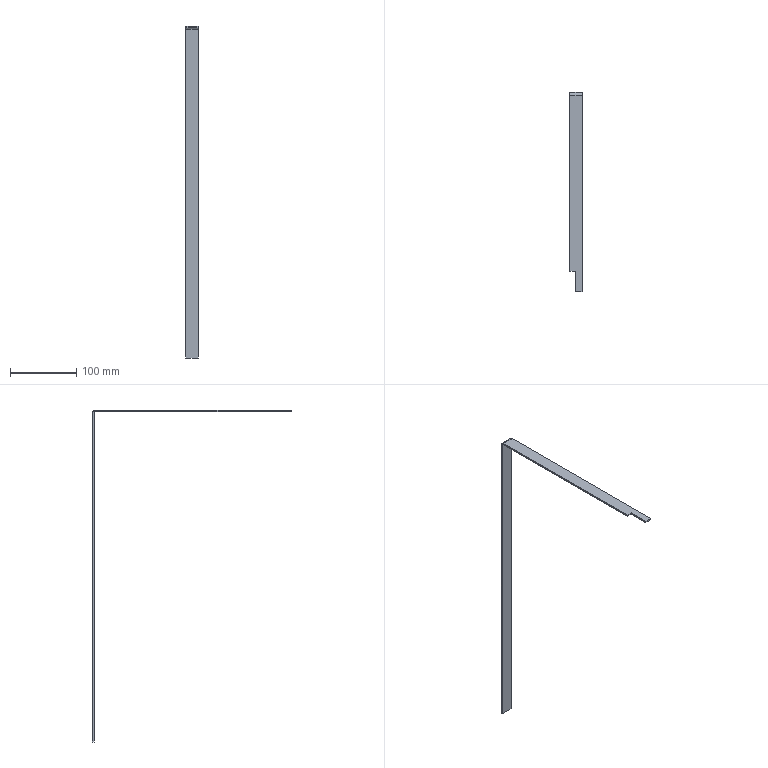Part | NX | features solid 2 | 1 solid | 12 faces | box 18.5 x 301.6 x 502.6 mm | volume 36384 mm3 | plane 10 | cylinder 2 | commonest cylinder face diameters 5 x1 10 x1
STEP:
#1=CARTESIAN_POINT('',(1098.,87.,522.6));
#2=VERTEX_POINT('',#1);
#3=CARTESIAN_POINT('',(1098.,87.,520.1));
#4=VERTEX_POINT('',#3);
#5=CARTESIAN_POINT('',(1098.,87.,520.1));
#6=DIRECTION('',(0.,0.,-1.));
#7=VECTOR('',#6,1000.);
#8=LINE('',#5,#7);
#9=EDGE_CURVE('',#2,#4,#8,.T.);
#10=ORIENTED_EDGE('',*,*,#9,.T.);
#11=CARTESIAN_POINT('',(1098.,56.,520.1));
#12=VERTEX_POINT('',#11);
#13=CARTESIAN_POINT('',(1098.,72.,520.1));
#14=DIRECTION('',(0.,1.,0.));
#15=VECTOR('',#14,1000.);
#16=LINE('',#13,#15);
#17=EDGE_CURVE('',#12,#4,#16,.T.);
#18=ORIENTED_EDGE('',*,*,#17,.F.);
#19=CARTESIAN_POINT('',(1098.,56.,522.6));
#20=VERTEX_POINT('',#19);
#21=CARTESIAN_POINT('',(1098.,56.,520.1));
#22=DIRECTION('',(0.,0.,-1.));
#23=VECTOR('',#22,1000.);
#24=LINE('',#21,#23);
#25=EDGE_CURVE('',#20,#12,#24,.T.);
#26=ORIENTED_EDGE('',*,*,#25,.F.);
#27=CARTESIAN_POINT('',(1098.,72.,522.6));
#28=DIRECTION('',(0.,1.,0.));
#29=VECTOR('',#28,1000.);
#30=LINE('',#27,#29);
#31=EDGE_CURVE('',#20,#2,#30,.T.);
#32=ORIENTED_EDGE('',*,*,#31,.T.);
#33=EDGE_LOOP('',(#10,#18,#26,#32));
#34=FACE_BOUND('',#33,.T.);
#35=CARTESIAN_POINT('',(1098.,72.,520.1));
#36=DIRECTION('',(-1.,0.,0.));
#37=DIRECTION('',(0.,0.,1.));
#38=AXIS2_PLACEMENT_3D('',#35,#36,#37);
#39=PLANE('',#38);
#40=ADVANCED_FACE('',(#34),#39,.T.);
#41=CARTESIAN_POINT('',(1090.,87.,522.6));
#42=VERTEX_POINT('',#41);
#43=CARTESIAN_POINT('',(1090.,87.,520.1));
#44=VERTEX_POINT('',#43);
#45=CARTESIAN_POINT('',(1090.,87.,520.1));
#46=DIRECTION('',(0.,0.,-1.));
#47=VECTOR('',#46,1000.);
#48=LINE('',#45,#47);
#49=EDGE_CURVE('',#42,#44,#48,.T.);
#50=ORIENTED_EDGE('',*,*,#49,.T.);
#51=CARTESIAN_POINT('',(1090.,87.,520.1));
#52=DIRECTION('',(-1.,0.,0.));
#53=VECTOR('',#52,1000.);
#54=LINE('',#51,#53);
#55=EDGE_CURVE('',#4,#44,#54,.T.);
#56=ORIENTED_EDGE('',*,*,#55,.F.);
#57=ORIENTED_EDGE('',*,*,#9,.F.);
#58=CARTESIAN_POINT('',(1090.,87.,522.6));
#59=DIRECTION('',(-1.,0.,0.));
#60=VECTOR('',#59,1000.);
#61=LINE('',#58,#60);
#62=EDGE_CURVE('',#2,#42,#61,.T.);
#63=ORIENTED_EDGE('',*,*,#62,.T.);
#64=EDGE_LOOP('',(#50,#56,#57,#63));
#65=FACE_BOUND('',#64,.T.);
#66=CARTESIAN_POINT('',(1090.,87.,520.1));
#67=DIRECTION('',(0.,-1.,0.));
#68=DIRECTION('',(-1.,0.,0.));
#69=AXIS2_PLACEMENT_3D('',#66,#67,#68);
#70=PLANE('',#69);
#71=ADVANCED_FACE('',(#65),#70,.T.);
#72=CARTESIAN_POINT('',(1108.5,357.6,517.6));
#73=VERTEX_POINT('',#72);
#74=CARTESIAN_POINT('',(1108.5,357.6,20.));
#75=VERTEX_POINT('',#74);
#76=CARTESIAN_POINT('',(1108.5,357.6,520.1));
#77=DIRECTION('',(0.,0.,-1.));
#78=VECTOR('',#77,1000.);
#79=LINE('',#76,#78);
#80=EDGE_CURVE('',#73,#75,#79,.T.);
#81=ORIENTED_EDGE('',*,*,#80,.T.);
#82=CARTESIAN_POINT('',(1090.,357.6,20.));
#83=VERTEX_POINT('',#82);
#84=CARTESIAN_POINT('',(1090.,357.6,20.));
#85=DIRECTION('',(1.,0.,0.));
#86=VECTOR('',#85,1000.);
#87=LINE('',#84,#86);
#88=EDGE_CURVE('',#83,#75,#87,.T.);
#89=ORIENTED_EDGE('',*,*,#88,.F.);
#90=CARTESIAN_POINT('',(1090.,357.6,517.6));
#91=VERTEX_POINT('',#90);
#92=CARTESIAN_POINT('',(1090.,357.6,520.1));
#93=DIRECTION('',(0.,0.,-1.));
#94=VECTOR('',#93,1000.);
#95=LINE('',#92,#94);
#96=EDGE_CURVE('',#91,#83,#95,.T.);
#97=ORIENTED_EDGE('',*,*,#96,.F.);
#98=CARTESIAN_POINT('',(1090.,357.6,517.6));
#99=DIRECTION('',(1.,0.,0.));
#100=VECTOR('',#99,1000.);
#101=LINE('',#98,#100);
#102=EDGE_CURVE('',#91,#73,#101,.T.);
#103=ORIENTED_EDGE('',*,*,#102,.T.);
#104=EDGE_LOOP('',(#81,#89,#97,#103));
#105=FACE_BOUND('',#104,.T.);
#106=CARTESIAN_POINT('',(1090.,357.6,520.1));
#107=DIRECTION('',(0.,-1.,0.));
#108=DIRECTION('',(-1.,0.,0.));
#109=AXIS2_PLACEMENT_3D('',#106,#107,#108);
#110=PLANE('',#109);
#111=ADVANCED_FACE('',(#105),#110,.F.);
#112=CARTESIAN_POINT('',(1108.5,352.6,522.6));
#113=VERTEX_POINT('',#112);
#114=CARTESIAN_POINT('',(1108.5,352.6,517.6));
#115=DIRECTION('',(-1.,0.,0.));
#116=DIRECTION('',(0.,0.,-1.));
#117=AXIS2_PLACEMENT_3D('',#114,#115,#116);
#118=CIRCLE('',#117,5.);
#119=EDGE_CURVE('',#113,#73,#118,.T.);
#120=ORIENTED_EDGE('',*,*,#119,.T.);
#121=ORIENTED_EDGE('',*,*,#102,.F.);
#122=CARTESIAN_POINT('',(1090.,352.6,522.6));
#123=VERTEX_POINT('',#122);
#124=CARTESIAN_POINT('',(1090.,352.6,517.6));
#125=DIRECTION('',(-1.,0.,0.));
#126=DIRECTION('',(0.,0.,-1.));
#127=AXIS2_PLACEMENT_3D('',#124,#125,#126);
#128=CIRCLE('',#127,5.);
#129=EDGE_CURVE('',#123,#91,#128,.T.);
#130=ORIENTED_EDGE('',*,*,#129,.F.);
#131=CARTESIAN_POINT('',(1090.,352.6,522.6));
#132=DIRECTION('',(1.,0.,0.));
#133=VECTOR('',#132,1000.);
#134=LINE('',#131,#133);
#135=EDGE_CURVE('',#123,#113,#134,.T.);
#136=ORIENTED_EDGE('',*,*,#135,.T.);
#137=EDGE_LOOP('',(#120,#121,#130,#136));
#138=FACE_BOUND('',#137,.T.);
#139=CARTESIAN_POINT('',(1090.,352.6,517.6));
#140=DIRECTION('',(1.,0.,0.));
#141=DIRECTION('',(0.,0.,-1.));
#142=AXIS2_PLACEMENT_3D('',#139,#140,#141);
#143=CYLINDRICAL_SURFACE('',#142,5.);
#144=ADVANCED_FACE('',(#138),#143,.T.);
#145=CARTESIAN_POINT('',(1090.,72.,522.6));
#146=DIRECTION('',(0.,1.,0.));
#147=VECTOR('',#146,1000.);
#148=LINE('',#145,#147);
#149=EDGE_CURVE('',#42,#123,#148,.T.);
#150=ORIENTED_EDGE('',*,*,#149,.F.);
#151=ORIENTED_EDGE('',*,*,#62,.F.);
#152=ORIENTED_EDGE('',*,*,#31,.F.);
#153=CARTESIAN_POINT('',(1108.5,56.,522.6));
#154=VERTEX_POINT('',#153);
#155=CARTESIAN_POINT('',(1090.,56.,522.6));
#156=DIRECTION('',(1.,0.,0.));
#157=VECTOR('',#156,1000.);
#158=LINE('',#155,#157);
#159=EDGE_CURVE('',#20,#154,#158,.T.);
#160=ORIENTED_EDGE('',*,*,#159,.T.);
#161=CARTESIAN_POINT('',(1108.5,72.,522.6));
#162=DIRECTION('',(0.,1.,0.));
#163=VECTOR('',#162,1000.);
#164=LINE('',#161,#163);
#165=EDGE_CURVE('',#154,#113,#164,.T.);
#166=ORIENTED_EDGE('',*,*,#165,.T.);
#167=ORIENTED_EDGE('',*,*,#135,.F.);
#168=EDGE_LOOP('',(#150,#151,#152,#160,#166,#167));
#169=FACE_BOUND('',#168,.T.);
#170=CARTESIAN_POINT('',(1090.,72.,522.6));
#171=DIRECTION('',(0.,0.,-1.));
#172=DIRECTION('',(-1.,0.,0.));
#173=AXIS2_PLACEMENT_3D('',#170,#171,#172);
#174=PLANE('',#173);
#175=ADVANCED_FACE('',(#169),#174,.F.);
#176=CARTESIAN_POINT('',(1108.5,355.1,517.6));
#177=VERTEX_POINT('',#176);
#178=CARTESIAN_POINT('',(1108.5,355.1,20.));
#179=VERTEX_POINT('',#178);
#180=CARTESIAN_POINT('',(1108.5,355.1,520.1));
#181=DIRECTION('',(0.,0.,-1.));
#182=VECTOR('',#181,1000.);
#183=LINE('',#180,#182);
#184=EDGE_CURVE('',#177,#179,#183,.T.);
#185=ORIENTED_EDGE('',*,*,#184,.F.);
#186=CARTESIAN_POINT('',(1090.,355.1,517.6));
#187=VERTEX_POINT('',#186);
#188=CARTESIAN_POINT('',(1090.,355.1,517.6));
#189=DIRECTION('',(1.,0.,0.));
#190=VECTOR('',#189,1000.);
#191=LINE('',#188,#190);
#192=EDGE_CURVE('',#187,#177,#191,.T.);
#193=ORIENTED_EDGE('',*,*,#192,.F.);
#194=CARTESIAN_POINT('',(1090.,355.1,20.));
#195=VERTEX_POINT('',#194);
#196=CARTESIAN_POINT('',(1090.,355.1,520.1));
#197=DIRECTION('',(0.,0.,-1.));
#198=VECTOR('',#197,1000.);
#199=LINE('',#196,#198);
#200=EDGE_CURVE('',#187,#195,#199,.T.);
#201=ORIENTED_EDGE('',*,*,#200,.T.);
#202=CARTESIAN_POINT('',(1090.,355.1,20.));
#203=DIRECTION('',(1.,0.,0.));
#204=VECTOR('',#203,1000.);
#205=LINE('',#202,#204);
#206=EDGE_CURVE('',#195,#179,#205,.T.);
#207=ORIENTED_EDGE('',*,*,#206,.T.);
#208=EDGE_LOOP('',(#185,#193,#201,#207));
#209=FACE_BOUND('',#208,.T.);
#210=CARTESIAN_POINT('',(1090.,355.1,520.1));
#211=DIRECTION('',(0.,-1.,0.));
#212=DIRECTION('',(-1.,0.,0.));
#213=AXIS2_PLACEMENT_3D('',#210,#211,#212);
#214=PLANE('',#213);
#215=ADVANCED_FACE('',(#209),#214,.T.);
#216=CARTESIAN_POINT('',(1108.5,352.6,520.1));
#217=VERTEX_POINT('',#216);
#218=CARTESIAN_POINT('',(1108.5,352.6,517.6));
#219=DIRECTION('',(-1.,0.,0.));
#220=DIRECTION('',(0.,0.,-1.));
#221=AXIS2_PLACEMENT_3D('',#218,#219,#220);
#222=CIRCLE('',#221,2.5);
#223=EDGE_CURVE('',#217,#177,#222,.T.);
#224=ORIENTED_EDGE('',*,*,#223,.F.);
#225=CARTESIAN_POINT('',(1090.,352.6,520.1));
#226=VERTEX_POINT('',#225);
#227=CARTESIAN_POINT('',(1090.,352.6,520.1));
#228=DIRECTION('',(1.,0.,0.));
#229=VECTOR('',#228,1000.);
#230=LINE('',#227,#229);
#231=EDGE_CURVE('',#226,#217,#230,.T.);
#232=ORIENTED_EDGE('',*,*,#231,.F.);
#233=CARTESIAN_POINT('',(1090.,352.6,517.6));
#234=DIRECTION('',(-1.,0.,0.));
#235=DIRECTION('',(0.,0.,-1.));
#236=AXIS2_PLACEMENT_3D('',#233,#234,#235);
#237=CIRCLE('',#236,2.5);
#238=EDGE_CURVE('',#226,#187,#237,.T.);
#239=ORIENTED_EDGE('',*,*,#238,.T.);
#240=ORIENTED_EDGE('',*,*,#192,.T.);
#241=EDGE_LOOP('',(#224,#232,#239,#240));
#242=FACE_BOUND('',#241,.T.);
#243=CARTESIAN_POINT('',(1090.,352.6,517.6));
#244=DIRECTION('',(1.,0.,0.));
#245=DIRECTION('',(0.,0.,-1.));
#246=AXIS2_PLACEMENT_3D('',#243,#244,#245);
#247=CYLINDRICAL_SURFACE('',#246,2.5);
#248=ADVANCED_FACE('',(#242),#247,.F.);
#249=ORIENTED_EDGE('',*,*,#55,.T.);
#250=CARTESIAN_POINT('',(1090.,72.,520.1));
#251=DIRECTION('',(0.,1.,0.));
#252=VECTOR('',#251,1000.);
#253=LINE('',#250,#252);
#254=EDGE_CURVE('',#44,#226,#253,.T.);
#255=ORIENTED_EDGE('',*,*,#254,.T.);
#256=ORIENTED_EDGE('',*,*,#231,.T.);
#257=CARTESIAN_POINT('',(1108.5,56.,520.1));
#258=VERTEX_POINT('',#257);
#259=CARTESIAN_POINT('',(1108.5,72.,520.1));
#260=DIRECTION('',(0.,1.,0.));
#261=VECTOR('',#260,1000.);
#262=LINE('',#259,#261);
#263=EDGE_CURVE('',#258,#217,#262,.T.);
#264=ORIENTED_EDGE('',*,*,#263,.F.);
#265=CARTESIAN_POINT('',(1090.,56.,520.1));
#266=DIRECTION('',(1.,0.,0.));
#267=VECTOR('',#266,1000.);
#268=LINE('',#265,#267);
#269=EDGE_CURVE('',#12,#258,#268,.T.);
#270=ORIENTED_EDGE('',*,*,#269,.F.);
#271=ORIENTED_EDGE('',*,*,#17,.T.);
#272=EDGE_LOOP('',(#249,#255,#256,#264,#270,#271));
#273=FACE_BOUND('',#272,.T.);
#274=CARTESIAN_POINT('',(1090.,72.,520.1));
#275=DIRECTION('',(0.,0.,-1.));
#276=DIRECTION('',(-1.,0.,0.));
#277=AXIS2_PLACEMENT_3D('',#274,#275,#276);
#278=PLANE('',#277);
#279=ADVANCED_FACE('',(#273),#278,.T.);
#280=ORIENTED_EDGE('',*,*,#25,.T.);
#281=ORIENTED_EDGE('',*,*,#269,.T.);
#282=CARTESIAN_POINT('',(1108.5,56.,520.1));
#283=DIRECTION('',(0.,0.,-1.));
#284=VECTOR('',#283,1000.);
#285=LINE('',#282,#284);
#286=EDGE_CURVE('',#154,#258,#285,.T.);
#287=ORIENTED_EDGE('',*,*,#286,.F.);
#288=ORIENTED_EDGE('',*,*,#159,.F.);
#289=EDGE_LOOP('',(#280,#281,#287,#288));
#290=FACE_BOUND('',#289,.T.);
#291=CARTESIAN_POINT('',(1090.,56.,520.1));
#292=DIRECTION('',(0.,1.,0.));
#293=DIRECTION('',(1.,0.,0.));
#294=AXIS2_PLACEMENT_3D('',#291,#292,#293);
#295=PLANE('',#294);
#296=ADVANCED_FACE('',(#290),#295,.F.);
#297=ORIENTED_EDGE('',*,*,#263,.T.);
#298=ORIENTED_EDGE('',*,*,#223,.T.);
#299=ORIENTED_EDGE('',*,*,#184,.T.);
#300=CARTESIAN_POINT('',(1108.5,355.1,20.));
#301=DIRECTION('',(0.,-1.,0.));
#302=VECTOR('',#301,1000.);
#303=LINE('',#300,#302);
#304=EDGE_CURVE('',#75,#179,#303,.T.);
#305=ORIENTED_EDGE('',*,*,#304,.F.);
#306=ORIENTED_EDGE('',*,*,#80,.F.);
#307=ORIENTED_EDGE('',*,*,#119,.F.);
#308=ORIENTED_EDGE('',*,*,#165,.F.);
#309=ORIENTED_EDGE('',*,*,#286,.T.);
#310=EDGE_LOOP('',(#297,#298,#299,#305,#306,#307,#308,#309));
#311=FACE_BOUND('',#310,.T.);
#312=CARTESIAN_POINT('',(1108.5,72.,520.1));
#313=DIRECTION('',(-1.,0.,0.));
#314=DIRECTION('',(0.,0.,1.));
#315=AXIS2_PLACEMENT_3D('',#312,#313,#314);
#316=PLANE('',#315);
#317=ADVANCED_FACE('',(#311),#316,.F.);
#318=CARTESIAN_POINT('',(1090.,355.1,20.));
#319=DIRECTION('',(0.,-1.,0.));
#320=VECTOR('',#319,1000.);
#321=LINE('',#318,#320);
#322=EDGE_CURVE('',#83,#195,#321,.T.);
#323=ORIENTED_EDGE('',*,*,#322,.F.);
#324=ORIENTED_EDGE('',*,*,#88,.T.);
#325=ORIENTED_EDGE('',*,*,#304,.T.);
#326=ORIENTED_EDGE('',*,*,#206,.F.);
#327=EDGE_LOOP('',(#323,#324,#325,#326));
#328=FACE_BOUND('',#327,.T.);
#329=CARTESIAN_POINT('',(1090.,355.1,20.));
#330=DIRECTION('',(0.,0.,-1.));
#331=DIRECTION('',(-1.,0.,0.));
#332=AXIS2_PLACEMENT_3D('',#329,#330,#331);
#333=PLANE('',#332);
#334=ADVANCED_FACE('',(#328),#333,.T.);
#335=ORIENTED_EDGE('',*,*,#49,.F.);
#336=ORIENTED_EDGE('',*,*,#149,.T.);
#337=ORIENTED_EDGE('',*,*,#129,.T.);
#338=ORIENTED_EDGE('',*,*,#96,.T.);
#339=ORIENTED_EDGE('',*,*,#322,.T.);
#340=ORIENTED_EDGE('',*,*,#200,.F.);
#341=ORIENTED_EDGE('',*,*,#238,.F.);
#342=ORIENTED_EDGE('',*,*,#254,.F.);
#343=EDGE_LOOP('',(#335,#336,#337,#338,#339,#340,#341,#342));
#344=FACE_BOUND('',#343,.T.);
#345=CARTESIAN_POINT('',(1090.,355.1,520.1));
#346=DIRECTION('',(-1.,0.,0.));
#347=DIRECTION('',(0.,0.,1.));
#348=AXIS2_PLACEMENT_3D('',#345,#346,#347);
#349=PLANE('',#348);
#350=ADVANCED_FACE('',(#344),#349,.T.);
#351=CLOSED_SHELL('',(#40,#71,#111,#144,#175,#215,#248,#279,#296,#317,#334,#350));
#352=MANIFOLD_SOLID_BREP('',#351);
#353=(LENGTH_UNIT()NAMED_UNIT(*)SI_UNIT(.MILLI.,.METRE.));
#354=UNCERTAINTY_MEASURE_WITH_UNIT(LENGTH_MEASURE(0.00001),#353,'','');
#355=(NAMED_UNIT(*)PLANE_ANGLE_UNIT()SI_UNIT($,.RADIAN.));
#356=(NAMED_UNIT(*)SI_UNIT($,.STERADIAN.)SOLID_ANGLE_UNIT());
#357=(GEOMETRIC_REPRESENTATION_CONTEXT(3)GLOBAL_UNCERTAINTY_ASSIGNED_CONTEXT((#354))GLOBAL_UNIT_ASSIGNED_CONTEXT((#353,#355,#356))REPRESENTATION_CONTEXT('',''));
#358=ADVANCED_BREP_SHAPE_REPRESENTATION('',(#352),#357);